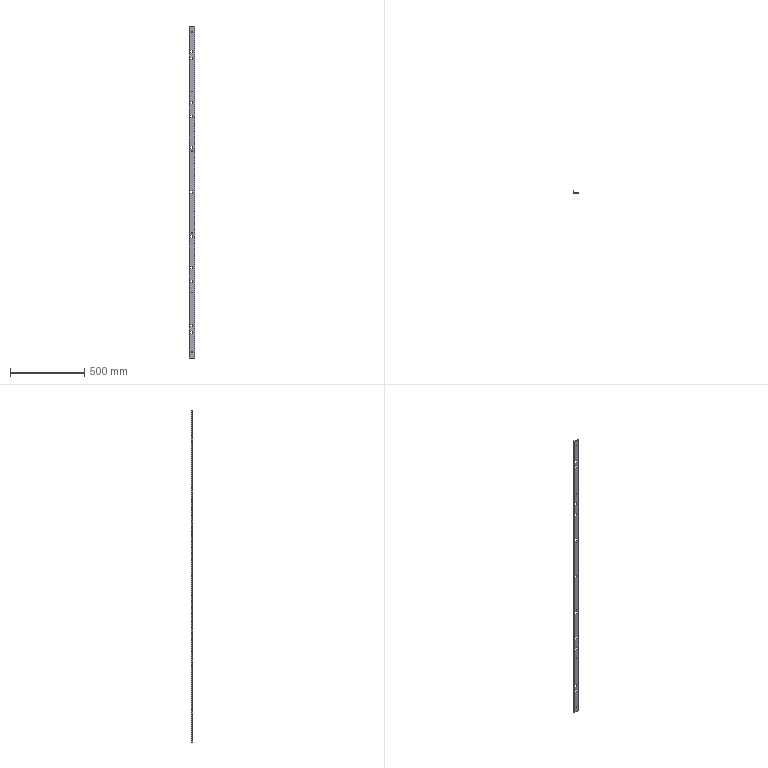Part | SolidWorks | features ICE 3, SMBaseFlange 2, FlatPattern 1, SheetMetal 1 | 1 solid | 235 faces | box 39 x 12 x 2234 mm | volume 207782 mm3 | plane 166 | cylinder 69 | commonest cylinder face diameters 5 x33 2 x12 6 x12 4.2 x10 4.5 x2